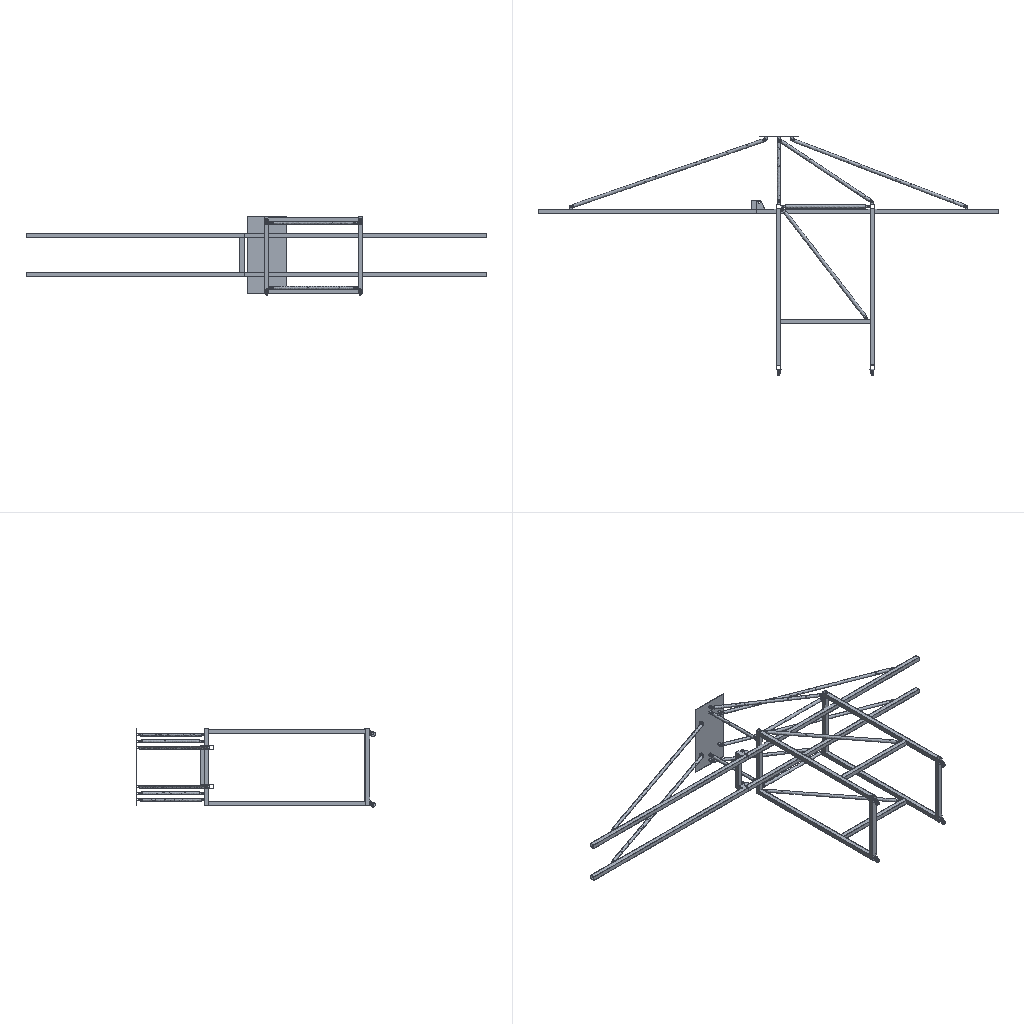Simulation study | ansys workbench
Ansys APDL input file, long lists of numbers shortened:
/batch
/config,noeldb,1     ! force off writing results to database
*get,_wallstrt,active,,time,wall
! ANSYS input file written by Workbench version 2021 R2
! File used for geometry attach:
/title,wbnew--____ (B5)
! ****** Begin Custom Load Command Snippet ******
/COM, ACT Extensions:
/COM,     LSDYNA, 2021.1
/COM,
! ****** End   Custom Load Command Snippet ******
*DIM,_wb_ProjectScratch_dir,string,248
_wb_ProjectScratch_dir(1) = ''
*DIM,_wb_SolverFiles_dir,string,248
_wb_SolverFiles_dir(1) = ''
*DIM,_wb_userfiles_dir,string,248
_wb_userfiles_dir(1) = ''
/com,--- Data in consistent NMM units. See Solving Units in the help system for more information.
/units,MPA
/nopr
/wb,file,start              !  signify a WB generated input file
/prep7
! Turn off shape checking because checks already performed inside WB mesher.
! See help system for more information.
SHPP,OFF,,NOWARN
/nolist
etcon,set             ! allow ANSYS to choose best KEYOP's for 180x elements, resets any applicable keyopt to MAPDL defaults
/com,*********** Nodes for the whole assembly ***********
nblock,3,,390517
(1i9,3e20.9e3)
   266169    -5.195703030E+03    -1.862202026E+01    -3.149999976E+02
! (355015 more lines like these left out)
-1
/com,*********** Nodes for all Remote Points ***********
nblock,3
(1i9,3e20.9e3)
   355017    -5.215703010E+03     1.837798024E+01     2.999999970E+02
! (51 more lines like these left out)
-1
/wb,elem,start            !  set before creation of elements
/com,*********** Elements for Body 1 "0314-02__\Mirror2" ***********
et,1,187
eblock,19,solid,,2767
(19i9)
        1        1        1        1        0        0        0        0       10        0        1      724      768      864      772     4690     4916     4696     4691
! (5533 more lines like these left out)
-1
/com,*********** Elements for Body 2 "0314-02__\Mirror2" ***********
et,2,187
eblock,19,solid,,3150
(19i9)
        2        2        2        2        0        0        0        0       10        0     2768     6049     6117     6205     6154    10579    10946    10584    10581
! (6299 more lines like these left out)
-1
/com,*********** Elements for Body 3 "0314-02__\Mirror2" ***********
et,3,187
eblock,19,solid,,2799
(19i9)
        3        3        3        3        0        0        0        0       10        0     5918    11222    11224    11223    11993    12731    12735    12730    12734
! (5597 more lines like these left out)
-1
/com,*********** Elements for Body 4 "0314-02__\Mirror2" ***********
et,4,187
eblock,19,solid,,3118
(19i9)
        4        4        4        4        0        0        0        0       10        0     8717    17274    17316    17360    17346    22036    22204    22040    22038
! (6235 more lines like these left out)
-1
/com,*********** Elements for Body 5 "Component5\NONE" ***********
et,5,187
eblock,19,solid,,15574
(19i9)
        5        5        5        5        0        0        0        0       10        0    11835    22268    22271    27204    27193    27612    27640    27616    27614
! (31147 more lines like these left out)
-1
! (75 more sections like these left out)
/wb,elem,end               !  done creating elements
/com,*********** Send User Defined Coordinate System(s) ***********
local,12,0,-5215.703,18.378,300.,-180.,0.,-180.
local,13,0,-5215.703,18.378,-300.,-180.,0.,-180.
local,14,0,-2224.364,1048.374,300.,-180.,0.,-180.
local,15,0,-2224.364,1048.374,-300.,-180.,0.,-180.
local,16,0,-2024.364,1048.374,500.,0.,0.,0.
local,17,0,-2024.364,1048.374,400.,0.,0.,0.
local,18,0,-1824.364,1048.374,-300.,-180.,0.,-180.
local,19,0,-2024.364,1048.374,-500.,0.,0.,0.
local,20,0,-2024.364,1048.374,-400.,0.,0.,0.
local,21,0,-1824.364,1048.374,300.,0.,0.,0.
local,22,0,-2024.364,88.374,-400.,0.,0.,0.
local,23,0,-2024.364,88.374,400.,0.,0.,0.
local,24,0,-589.842,91.993,500.,0.,0.,0.
local,25,0,-589.842,91.993,-500.,0.,0.,0.
local,26,0,858.879,18.378,300.,0.,0.,0.
local,27,0,858.879,18.378,-300.,-180.,0.,-180.
local,28,0,-2324.363,83.378,-300.,-180.,0.,-180.
local,29,0,-2324.363,83.378,300.,0.,0.,0.
local,30,0,-1954.364,21.954,500.,-180.,0.,-180.
local,31,0,-1954.364,21.954,-500.,0.,0.,0.
local,32,0,-1954.364,-32.126,-552.5,0.,0.,0.
local,33,0,-1954.364,-32.126,552.5,0.,0.,0.
local,34,0,-659.864,21.954,500.,-180.,0.,-180.
local,35,0,-659.864,21.954,-500.,0.,0.,0.
local,36,0,-689.364,-1677.626,-552.5,-180.,0.,-180.
local,37,0,-689.364,-1677.626,552.5,-180.,0.,-180.
csys,0
toffst,273.15,  ! Temperature offset from absolute zero
/com,*********** Set Reference Temperature ***********
tref,22.
/wb,mat,start              !  starting to send materials
/com,*********** Send Materials ***********
Temperature = 'TEMP' ! Temperature
MP,DENS,1,7.85e-09,	! tonne mm^-3
MP,ALPX,1,1.2e-05,	! C^-1
MP,C,1,434000000,	! mm^2 s^-2 C^-1
MP,KXX,1,60.5,	! tonne mm s^-3 C^-1
MP,RSVX,1,0.00017,	! ohm mm
MP,EX,1,200000,	! tonne s^-2 mm^-1
MP,NUXY,1,0.3,
MP,MURX,1,10000,
Temperature = 'TEMP' ! Temperature
MP,DENS,2,7.85e-09,	! tonne mm^-3
MP,ALPX,2,1.2e-05,	! C^-1
MP,C,2,434000000,	! mm^2 s^-2 C^-1
MP,KXX,2,60.5,	! tonne mm s^-3 C^-1
MP,RSVX,2,0.00017,	! ohm mm
MP,EX,2,200000,	! tonne s^-2 mm^-1
MP,NUXY,2,0.3,
MP,MURX,2,10000,
Temperature = 'TEMP' ! Temperature
MP,DENS,3,7.85e-09,	! tonne mm^-3
MP,ALPX,3,1.2e-05,	! C^-1
MP,C,3,434000000,	! mm^2 s^-2 C^-1
MP,KXX,3,60.5,	! tonne mm s^-3 C^-1
MP,RSVX,3,0.00017,	! ohm mm
MP,EX,3,200000,	! tonne s^-2 mm^-1
MP,NUXY,3,0.3,
MP,MURX,3,10000,
Temperature = 'TEMP' ! Temperature
MP,DENS,4,7.85e-09,	! tonne mm^-3
MP,ALPX,4,1.2e-05,	! C^-1
MP,C,4,434000000,	! mm^2 s^-2 C^-1
MP,KXX,4,60.5,	! tonne mm s^-3 C^-1
MP,RSVX,4,0.00017,	! ohm mm
MP,EX,4,200000,	! tonne s^-2 mm^-1
MP,NUXY,4,0.3,
MP,MURX,4,10000,
Temperature = 'TEMP' ! Temperature
MP,DENS,5,7.85e-09,	! tonne mm^-3
MP,ALPX,5,1.2e-05,	! C^-1
MP,C,5,434000000,	! mm^2 s^-2 C^-1
MP,KXX,5,60.5,	! tonne mm s^-3 C^-1
MP,RSVX,5,0.00017,	! ohm mm
MP,EX,5,200000,	! tonne s^-2 mm^-1
MP,NUXY,5,0.3,
MP,MURX,5,10000,
Temperature = 'TEMP' ! Temperature
MP,DENS,6,7.85e-09,	! tonne mm^-3
MP,ALPX,6,1.2e-05,	! C^-1
MP,C,6,434000000,	! mm^2 s^-2 C^-1
MP,KXX,6,60.5,	! tonne mm s^-3 C^-1
MP,RSVX,6,0.00017,	! ohm mm
MP,EX,6,200000,	! tonne s^-2 mm^-1
MP,NUXY,6,0.3,
MP,MURX,6,10000,
Temperature = 'TEMP' ! Temperature
MP,DENS,7,7.85e-09,	! tonne mm^-3
MP,ALPX,7,1.2e-05,	! C^-1
MP,C,7,434000000,	! mm^2 s^-2 C^-1
MP,KXX,7,60.5,	! tonne mm s^-3 C^-1
MP,RSVX,7,0.00017,	! ohm mm
MP,EX,7,200000,	! tonne s^-2 mm^-1
MP,NUXY,7,0.3,
MP,MURX,7,10000,
Temperature = 'TEMP' ! Temperature
MP,DENS,8,7.85e-09,	! tonne mm^-3
MP,ALPX,8,1.2e-05,	! C^-1
MP,C,8,434000000,	! mm^2 s^-2 C^-1
MP,KXX,8,60.5,	! tonne mm s^-3 C^-1
MP,RSVX,8,0.00017,	! ohm mm
MP,EX,8,200000,	! tonne s^-2 mm^-1
MP,NUXY,8,0.3,
MP,MURX,8,10000,
Temperature = 'TEMP' ! Temperature
MP,DENS,9,7.85e-09,	! tonne mm^-3
MP,ALPX,9,1.2e-05,	! C^-1
MP,C,9,434000000,	! mm^2 s^-2 C^-1
MP,KXX,9,60.5,	! tonne mm s^-3 C^-1
MP,RSVX,9,0.00017,	! ohm mm
MP,EX,9,200000,	! tonne s^-2 mm^-1
! (641 more lines like these left out)
/wb,mat,end                !  done sending materials
/com,*********** Send Sheet Properties ***********
sectype,44,shell
secdata,4.
secoff,mid
sectype,45,shell
secdata,4.
secoff,mid
sectype,46,shell
secdata,4.
secoff,mid
sectype,47,shell
secdata,4.
secoff,mid
sectype,48,shell
secdata,4.
secoff,mid
sectype,49,shell
secdata,10.
secoff,mid
sectype,50,shell
secdata,10.
secoff,mid
sectype,51,shell
secdata,10.
secoff,mid
sectype,52,shell
secdata,10.
secoff,mid
sectype,53,shell
secdata,4.
secoff,mid
sectype,54,shell
secdata,4.
secoff,mid
sectype,55,shell
secdata,10.
secoff,mid
sectype,56,shell
secdata,10.
secoff,mid
sectype,57,shell
secdata,10.
secoff,mid
sectype,58,shell
secdata,10.
secoff,mid
sectype,59,shell
secdata,10.
secoff,mid
sectype,60,shell
secdata,10.
secoff,mid
sectype,61,shell
secdata,10.
secoff,mid
sectype,62,shell
secdata,10.
secoff,mid
sectype,63,shell
secdata,4.
secoff,mid
sectype,64,shell
secdata,4.
secoff,mid
sectype,65,shell
secdata,4.
secoff,mid
sectype,66,shell
secdata,4.
secoff,mid
sectype,67,shell
secdata,4.
secoff,mid
sectype,68,shell
secdata,4.
secoff,mid
sectype,69,shell
secdata,4.
secoff,mid
sectype,70,shell
! (96 more lines like these left out)
/wb,contact,start          !  starting to send contact
/com,*********** Create Contact "接触区域" ***********
/com,            Real Constant Set For Above Contact Is 82 & 81
*set,tid,82
*set,cid,81
r,tid
r,cid
et,tid,170
et,cid,174
eblock,10,,,515
(15i9)
   306121       82       82       82        0       10       15       16       16      961     1003       16      962
! (514 more lines like these left out)
-1
eblock,10,,,515
(15i9)
   306636       81       81       81        0       10       15       16       16      961     1003       16      962
! (514 more lines like these left out)
-1
eblock,10,,,119
(15i9)
   307151       81       82       81        0   337162   337163   337171   337170
! (118 more lines like these left out)
-1
eblock,10,,,119
(15i9)
   307270       82       81       82        0   337162   337163   337171   337170
! (118 more lines like these left out)
-1
keyo,cid,8,2               ! auto create asymmetric contact (from Program Controlled setting)
keyo,cid,10,0              ! adjust contact stiffness each NR iteration (from Program Controlled setting)
keyo,cid,12,5              ! bonded always
keyo,cid,18,1              ! small sliding turned on by application
keyo,cid,2,0               ! augmented Lagrange (from Program Controlled setting)
keyo,cid,4,0               ! on Gauss point (from Program Controlled setting)
keyo,cid,9,1               ! ignore initial gaps/penetration
keyo,cid,7,0               ! No Prediction
rmod,tid,3,10.      ! FKN
rmod,tid,5,0.       ! ICONT
rmod,tid,6,-20.121  ! PINB
rmod,tid,10,0.      ! CNOF
rmod,tid,12,0.      ! FKT
rmod,tid,36,721     ! WB DSID
rmod,cid,3,10.      ! FKN
rmod,cid,5,0.       ! ICONT
rmod,cid,6,-20.121  ! PINB
rmod,cid,10,0.      ! CNOF
rmod,cid,12,0.      ! FKT
rmod,cid,36,721     ! WB DSID
/com,*********** Create Contact "接触区域 2" ***********
/com,            Real Constant Set For Above Contact Is 84 & 83
*set,tid,84
*set,cid,83
r,tid
r,cid
et,tid,170
et,cid,174
eblock,10,,,511
(15i9)
   307389       84       84       84        0     5728     5249     5264     5264     6318     6314     5264     6426
! (510 more lines like these left out)
-1
eblock,10,,,511
(15i9)
   307900       83       83       83        0     5728     5249     5264     5264     6318     6314     5264     6426
! (510 more lines like these left out)
-1
eblock,10,,,98
(15i9)
   308411       83       84       83        0   332618   334222   334224   334223
! (97 more lines like these left out)
-1
eblock,10,,,98
(15i9)
   308509       84       83       84        0   332618   334222   334224   334223
! (97 more lines like these left out)
-1
keyo,cid,8,2               ! auto create asymmetric contact (from Program Controlled setting)
keyo,cid,10,0              ! adjust contact stiffness each NR iteration (from Program Controlled setting)
keyo,cid,12,5              ! bonded always
keyo,cid,18,1              ! small sliding turned on by application
keyo,cid,2,0               ! augmented Lagrange (from Program Controlled setting)
keyo,cid,4,0               ! on Gauss point (from Program Controlled setting)
keyo,cid,9,1               ! ignore initial gaps/penetration
keyo,cid,7,0               ! No Prediction
rmod,tid,3,10.      ! FKN
rmod,tid,5,0.       ! ICONT
rmod,tid,6,-20.121  ! PINB
rmod,tid,10,0.      ! CNOF
rmod,tid,12,0.      ! FKT
rmod,tid,36,724     ! WB DSID
rmod,cid,3,10.      ! FKN
rmod,cid,5,0.       ! ICONT
rmod,cid,6,-20.121  ! PINB
rmod,cid,10,0.      ! CNOF
rmod,cid,12,0.      ! FKT
rmod,cid,36,724     ! WB DSID
/com,*********** Create Contact "接触区域 3" ***********
/com,            Real Constant Set For Above Contact Is 86 & 85
*set,tid,86
*set,cid,85
r,tid
r,cid
et,tid,170
et,cid,174
eblock,10,,,509
(15i9)
   308607       86       86       86        0    11138    11617    11149    11149    12120    12195    11149    12113
! (508 more lines like these left out)
-1
eblock,10,,,509
(15i9)
   309116       85       85       85        0    11138    11617    11149    11149    12120    12195    11149    12113
! (508 more lines like these left out)
-1
eblock,10,,,119
(15i9)
   309625       85       86       85        0   321316   321317   321319   321318
! (118 more lines like these left out)
-1
eblock,10,,,119
(15i9)
   309744       86       85       86        0   321316   321317   321319   321318
! (118 more lines like these left out)
-1
keyo,cid,8,2               ! auto create asymmetric contact (from Program Controlled setting)
keyo,cid,10,0              ! adjust contact stiffness each NR iteration (from Program Controlled setting)
keyo,cid,12,5              ! bonded always
keyo,cid,18,1              ! small sliding turned on by application
keyo,cid,2,0               ! augmented Lagrange (from Program Controlled setting)
keyo,cid,4,0               ! on Gauss point (from Program Controlled setting)
keyo,cid,9,1               ! ignore initial gaps/penetration
keyo,cid,7,0               ! No Prediction
rmod,tid,3,10.      ! FKN
rmod,tid,5,0.       ! ICONT
rmod,tid,6,-20.121  ! PINB
rmod,tid,10,0.      ! CNOF
rmod,tid,12,0.      ! FKT
rmod,tid,36,727     ! WB DSID
rmod,cid,3,10.      ! FKN
rmod,cid,5,0.       ! ICONT
rmod,cid,6,-20.121  ! PINB
rmod,cid,10,0.      ! CNOF
rmod,cid,12,0.      ! FKT
rmod,cid,36,727     ! WB DSID
/com,*********** Create Contact "接触区域 4" ***********
/com,            Real Constant Set For Above Contact Is 88 & 87
*set,tid,88
*set,cid,87
r,tid
r,cid
et,tid,170
et,cid,174
eblock,10,,,511
(15i9)
   309863       88       88       88        0    16417    16896    16428    16428    17486    17561    16428    17480
! (510 more lines like these left out)
-1
eblock,10,,,511
(15i9)
   310374       87       87       87        0    16417    16896    16428    16428    17486    17561    16428    17480
! (510 more lines like these left out)
-1
eblock,10,,,98
(15i9)
   310885       87       88       87        0   321252   321253   321255   321254
! (97 more lines like these left out)
-1
eblock,10,,,98
(15i9)
   310983       88       87       88        0   321252   321253   321255   321254
! (97 more lines like these left out)
-1
keyo,cid,8,2               ! auto create asymmetric contact (from Program Controlled setting)
keyo,cid,10,0              ! adjust contact stiffness each NR iteration (from Program Controlled setting)
keyo,cid,12,5              ! bonded always
keyo,cid,18,1              ! small sliding turned on by application
keyo,cid,2,0               ! augmented Lagrange (from Program Controlled setting)
keyo,cid,4,0               ! on Gauss point (from Program Controlled setting)
keyo,cid,9,1               ! ignore initial gaps/penetration
keyo,cid,7,0               ! No Prediction
rmod,tid,3,10.      ! FKN
rmod,tid,5,0.       ! ICONT
rmod,tid,6,-20.121  ! PINB
rmod,tid,10,0.      ! CNOF
rmod,tid,12,0.      ! FKT
rmod,tid,36,730     ! WB DSID
rmod,cid,3,10.      ! FKN
rmod,cid,5,0.       ! ICONT
rmod,cid,6,-20.121  ! PINB
rmod,cid,10,0.      ! CNOF
rmod,cid,12,0.      ! FKT
rmod,cid,36,730     ! WB DSID
/com,*********** Create Contact "接触区域" ***********
/com,            Real Constant Set For Above Contact Is 90 & 89
*set,tid,90
*set,cid,89
r,tid
r,cid
et,tid,170
et,cid,174
eblock,10,,,12
(15i9)
   311081       90       90       90        0   255665   255666   255579   255585   255992   255819   255818   255831
! (11 more lines like these left out)
-1
eblock,10,,,12
(15i9)
   311093       89       89       89        0   255665   255666   255579   255585   255992   255819   255818   255831
! (11 more lines like these left out)
-1
eblock,10,,,69
(15i9)
   311105       89       90       89        0   353611   353609   353605   353606
! (68 more lines like these left out)
-1
eblock,10,,,69
(15i9)
   311174       90       89       90        0   353611   353609   353605   353606
! (68 more lines like these left out)
-1
keyo,cid,8,2               ! auto create asymmetric contact (from Program Controlled setting)
keyo,cid,10,0              ! adjust contact stiffness each NR iteration (from Program Controlled setting)
keyo,cid,12,5              ! bonded always
keyo,cid,18,1              ! small sliding turned on by application
keyo,cid,2,0               ! augmented Lagrange (from Program Controlled setting)
keyo,cid,4,0               ! on Gauss point (from Program Controlled setting)
keyo,cid,9,1               ! ignore initial gaps/penetration
keyo,cid,7,0               ! No Prediction
rmod,tid,3,10.      ! FKN
rmod,tid,5,0.       ! ICONT
rmod,tid,6,-20.121  ! PINB
rmod,tid,10,0.      ! CNOF
rmod,tid,12,0.      ! FKT
rmod,tid,36,735     ! WB DSID
rmod,cid,3,10.      ! FKN
rmod,cid,5,0.       ! ICONT
rmod,cid,6,-20.121  ! PINB
rmod,cid,10,0.      ! CNOF
rmod,cid,12,0.      ! FKT
rmod,cid,36,735     ! WB DSID
! (15 more sections like these left out)
/wb,contact,end            !  done creating contacts
/golist
/wb,load,start             !  starting to send loads
/com,*********** Fixed Supports ***********
CMBLOCK,_FIXEDSU,NODE,      960
(8i10)
       154       155       156       157       158       159       160       161
! (119 more lines like these left out)
cmsel,s,_FIXEDSU
d,all,all
nsel,all
/com,*********** Create Remote Point "内部远程点" ***********
! -------- Remote Point Used by "回转 - Component6\NONE 至 多个" --------
*set,tid,122
*set,cid,121
et,cid,174
et,tid,170
keyo,tid,2,1               ! Don't fix the pilot node
keyo,tid,4,111111
keyo,cid,12,5              ! Bonded Contact
keyo,cid,4,2               ! Rigid CERIG style load
keyo,cid,2,2               ! MPC style contact
eblock,10,,,14
(15i9)
   314905      121      121      121        0    53421    53420    58349    58349    58828    58833    58349    58839
! (13 more lines like these left out)
-1
*set,_npilot,355017
_npilot456=_npilot
type,tid
mat ,cid
real,cid
tshape,pilo
en,314919,_npilot
tshape
csys,12
nrot,355017
csys,0
/com,*********** Create Remote Point "内部远程点 2" ***********
! -------- Remote Point Used by "回转 - Component6\NONE 至 多个" --------
*set,tid,124
*set,cid,123
et,cid,175
et,tid,170
keyo,tid,2,1               ! Don't fix the pilot node
keyo,tid,4,111111
keyo,cid,12,5              ! Bonded Contact
keyo,cid,4,0               ! Rigid CERIG style load
keyo,cid,2,2               ! MPC style contact
mat,123
real,123
type,123
en,314920,274073
en,314921,274078
en,314922,274079
en,314923,274085
en,314924,274086
en,314925,274088
en,314926,274099
en,314927,274101
en,314928,274103
en,314929,274104
en,314930,274107
en,314931,274108
en,314932,274111
en,314933,274115
en,314934,274117
en,314935,274123
*set,_npilot,355018
_npilot457=_npilot
type,tid
mat ,cid
real,cid
tshape,pilo
en,314936,_npilot
tshape
csys,12
nrot,355018
csys,0
/com,*********** Create Remote Point "内部远程点 3" ***********
! -------- Remote Point Used by "回转 - Component5\NONE 至 多个" --------
*set,tid,126
*set,cid,125
et,cid,174
et,tid,170
keyo,tid,2,1               ! Don't fix the pilot node
keyo,tid,4,111111
keyo,cid,12,5              ! Bonded Contact
keyo,cid,4,2               ! Rigid CERIG style load
keyo,cid,2,2               ! MPC style contact
eblock,10,,,14
(15i9)
   314937      125      125      125        0    22274    22273    27189    27189    27653    27658    27189    27664
! (13 more lines like these left out)
-1
*set,_npilot,355019
_npilot460=_npilot
type,tid
mat ,cid
real,cid
tshape,pilo
en,314951,_npilot
tshape
csys,13
nrot,355019
csys,0
/com,*********** Create Remote Point "内部远程点 4" ***********
! -------- Remote Point Used by "回转 - Component5\NONE 至 多个" --------
*set,tid,128
*set,cid,127
et,cid,175
et,tid,170
keyo,tid,2,1               ! Don't fix the pilot node
keyo,tid,4,111111
keyo,cid,12,5              ! Bonded Contact
keyo,cid,4,0               ! Rigid CERIG style load
keyo,cid,2,2               ! MPC style contact
mat,127
real,127
type,127
en,314952,280176
en,314953,280177
en,314954,280180
en,314955,280181
en,314956,280184
en,314957,280188
en,314958,280190
en,314959,280196
en,314960,282259
en,314961,282264
en,314962,282265
en,314963,282271
en,314964,282272
en,314965,282274
en,314966,282285
en,314967,282287
*set,_npilot,355020
_npilot461=_npilot
type,tid
mat ,cid
real,cid
tshape,pilo
en,314968,_npilot
tshape
csys,13
nrot,355020
csys,0
/com,*********** Create Remote Point "内部远程点 5" ***********
! -------- Remote Point Used by "回转 - Component6\NONE 至 多个" --------
*set,tid,130
*set,cid,129
et,cid,174
et,tid,170
keyo,tid,2,1               ! Don't fix the pilot node
keyo,tid,4,111111
keyo,cid,12,5              ! Bonded Contact
keyo,cid,4,2               ! Rigid CERIG style load
keyo,cid,2,2               ! MPC style contact
eblock,10,,,16
(15i9)
   314969      129      129      129        0    58354    53412    58355    58355    58770    58771    58355    84613
! (15 more lines like these left out)
-1
*set,_npilot,355021
_npilot464=_npilot
type,tid
mat ,cid
real,cid
tshape,pilo
en,314985,_npilot
tshape
csys,14
nrot,355021
csys,0
! (47 more sections like these left out)
/com,*********** Create Joint "回转 - Component6\NONE 至 多个" ***********
/com,            Real Constant Set For Above Joint Is 225
! Joint Element Type Declaration and Definition using MPC184
*set,_jid,225
et,_jid,184
keyo,_jid,1,6           ! Revolute Joint
keyo,_jid,4,1           ! Z Axis is revolute axis
sectype,_jid, joint, revo, _wbjoint
secjoint,,12,12
mat,_jid
real,_jid
type,_jid
secnum,_jid
en,306043,355017,355018      ! body to body joint
/com,*********** Create Joint "回转 - Component5\NONE 至 多个" ***********
/com,            Real Constant Set For Above Joint Is 226
! Joint Element Type Declaration and Definition using MPC184
*set,_jid,226
et,_jid,184
keyo,_jid,1,6           ! Revolute Joint
keyo,_jid,4,1           ! Z Axis is revolute axis
sectype,_jid, joint, revo, _wbjoint
secjoint,,13,13
mat,_jid
real,_jid
type,_jid
secnum,_jid
en,306044,355019,355020      ! body to body joint
/com,*********** Create Joint "回转 - Component6\NONE 至 多个" ***********
/com,            Real Constant Set For Above Joint Is 227
! Joint Element Type Declaration and Definition using MPC184
*set,_jid,227
et,_jid,184
keyo,_jid,1,6           ! Revolute Joint
keyo,_jid,4,1           ! Z Axis is revolute axis
sectype,_jid, joint, revo, _wbjoint
secjoint,,14,14
mat,_jid
real,_jid
type,_jid
secnum,_jid
en,306045,355021,355022      ! body to body joint
/com,*********** Create Joint "回转 - Component5\NONE 至 多个" ***********
/com,            Real Constant Set For Above Joint Is 228
! Joint Element Type Declaration and Definition using MPC184
*set,_jid,228
et,_jid,184
keyo,_jid,1,6           ! Revolute Joint
keyo,_jid,4,1           ! Z Axis is revolute axis
sectype,_jid, joint, revo, _wbjoint
secjoint,,15,15
mat,_jid
real,_jid
type,_jid
secnum,_jid
en,306046,355023,355024      ! body to body joint
/com,*********** Create Joint "回转 - Component16\NONE 至 多个" ***********
/com,            Real Constant Set For Above Joint Is 229
! Joint Element Type Declaration and Definition using MPC184
*set,_jid,229
et,_jid,184
keyo,_jid,1,6           ! Revolute Joint
keyo,_jid,4,1           ! Z Axis is revolute axis
sectype,_jid, joint, revo, _wbjoint
secjoint,,16,16
mat,_jid
real,_jid
type,_jid
secnum,_jid
en,306047,355025,355026      ! body to body joint
! (21 more sections like these left out)
/com,*********** Define Force Using Surface Effect Elements ***********
local,38,0,0.,0.,0.,0.,0.,0.
csys,0
et,251,154
eblock,10,,,9834
(15i9)
   315799      251      251      251       38   284490   284489   284507   284507
! (9833 more lines like these left out)
-1
esel,s,type,,251
keyop,251,2,1                ! Apply load in local coordinate system
keyop,251,7,1                ! Use original area so load is constant in large deformation
esel,all
/gst,on,on
fini
*get,_numnode,node,0,count
*get,_numelem,elem,0,count
*get, _MAXELEMNUM, elem, 0, NUM, MAX
*get, _MAXNODENUM, node, 0, NUM, MAX
*get, _MAXELEMTYPE, etyp, 0, NUM, MAX
*get, _MAXREALCONST, real, 0, NUM, MAX
/go
/wb,load,end               !  done creating loads
/com,--- Number of total nodes = %_numnode%
/com,--- Number of contact elements = 19460
/com,--- Number of spring elements = 0
/com,--- Number of bearing elements = 0
/com,--- Number of solid elements = 229058
/com,--- Number of condensed parts = 0
/com,--- Number of total elements = %_numelem%
*get,_wallbsol,active,,time,wall
/com,****************************************************************************
/com,*************************    SOLUTION       ********************************
/com,****************************************************************************
/solu
antype,0                   ! static analysis
_thickRatio=0.4     ! Ratio of thick parts in the model
eqsl,sparse,,,,,1
cntr,print,1               ! print out contact info and also make no initial contact an error
dmpoption,emat,no             ! Don't combine emat file for DANSYS
dmpoption,esav,no             ! Don't combine esav file for DANSYS
nldiag,cont,iter           ! print out contact info each equilibrium iteration
rescontrol,,none                 ! Do not keep any restart files
/com,****************************************************
/com,******************* SOLVE FOR LS 1 OF 1 ****************
esel,s,type,,251
nsle
sfe,all,1,pres,1,0.
sfe,all,2,pres,1,-1.08504117672947e-002
sfe,all,3,pres,1,0.
nsel,all
esel,all
/nopr
/gopr
nsub,1,1,1
time,1.
outres,erase
outres,all,none
outres,nsol,all,
outres,rsol,all
outres,eangl,all
outres,etmp,all
outres,veng,all
outres,strs,all,
outres,epel,all,
outres,eppl,all,
outres,cont,all,
/nopr
esel,s,type,,225
esel,a,type,,226,250
cm,_elmisc,elem
esel,all
/gopr
outres,misc,all,_elmisc
! *********** WB SOLVE COMMAND ***********
! check interactive state
*get,ANSINTER_,active,,int
*if,ANSINTER_,ne,0,then
/eof
*endif
solve
/com *************** Write FE CONNECTORS *********
CEWRITE,file,ce,,INTE
/com,****************************************************
/com,*************** FINISHED SOLVE FOR LS 1 *************
*get,_wallasol,active,,time,wall
/nopr
*get,_numnode,node,0,count
*get,_numelem,elem,0,count
*get, _MAXELEMNUM, elem, 0, NUM, MAX
*get, _MAXNODENUM, node, 0, NUM, MAX,,,INTERNAL
*get, _MAXELEMTYPE, etyp, 0, NUM, MAX
*get, _MAXREALCONST, real, 0, NUM, MAX
/gopr
/post1
xmlo,ENCODING,ISO-8859-1
xmlo,parm
/xml,parm,xml
fini
/gopr
*get,_walldone,active,,time,wall
_preptime=(_wallbsol-_wallstrt)*3600
_solvtime=(_wallasol-_wallbsol)*3600
_posttime=(_walldone-_wallasol)*3600
_totaltim=(_walldone-_wallstrt)*3600
*get,_dlbratio,active,0,solu,dlbr
*get,_combtime,active,0,solu,comb
*get,_ssmode,active,0,solu,ssmm
*get,_ndofs,active,0,solu,ndof
/com,--- Total number of nodes = %_numnode%
/com,--- Total number of elements = %_numelem%
/com,--- Element load balance ratio = %_dlbratio%
/com,--- Time to combine distributed files = %_combtime%
/com,--- Sparse memory mode = %_ssmode%
/com,--- Number of DOF = %_ndofs%
/wb,file,end               ! done with WB generated input